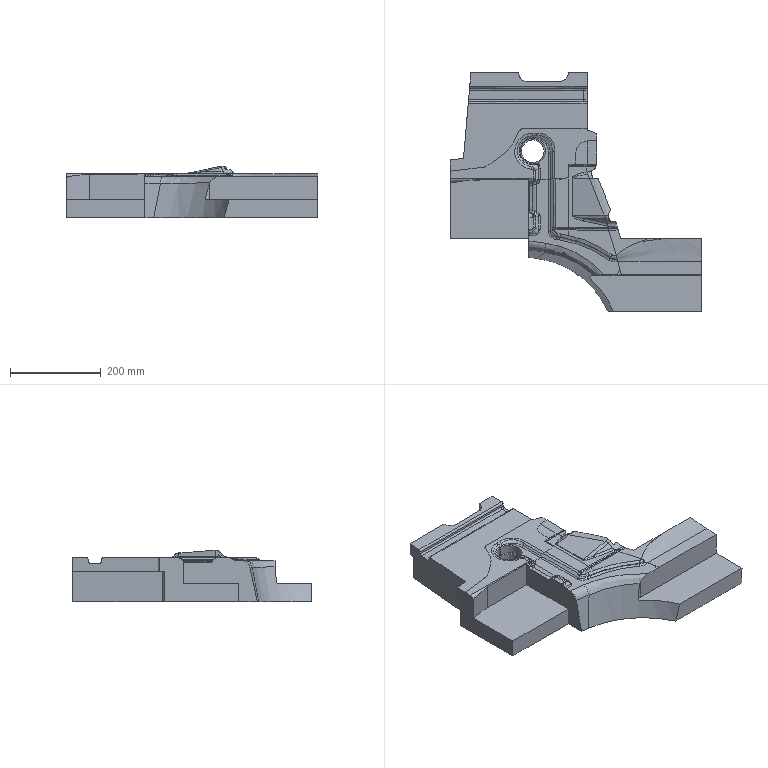Part | NX | features solid 2 | 1 solid | 183 faces | box 552.249 x 525 x 114.078 mm | volume 11768272 mm3 | spline 169 | plane 11 | cylinder 3 | commonest cylinder face diameters 40 x2 56 x1